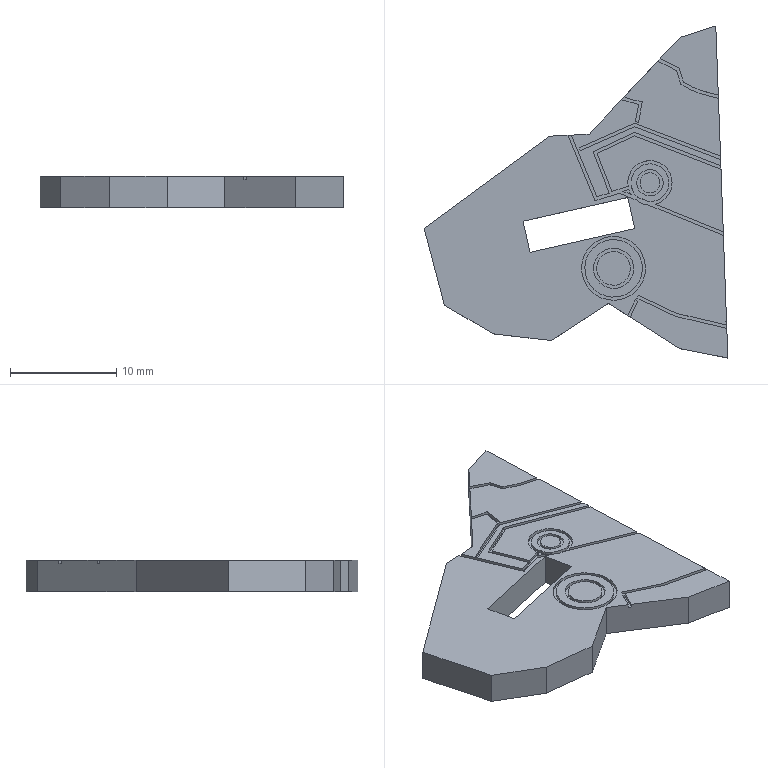Part | SolidWorks | features BaseBody 1 | 1 solid | 118 faces | box 28.584 x 31.242 x 3 mm | volume 1486 mm3 | plane 69 | spline 49